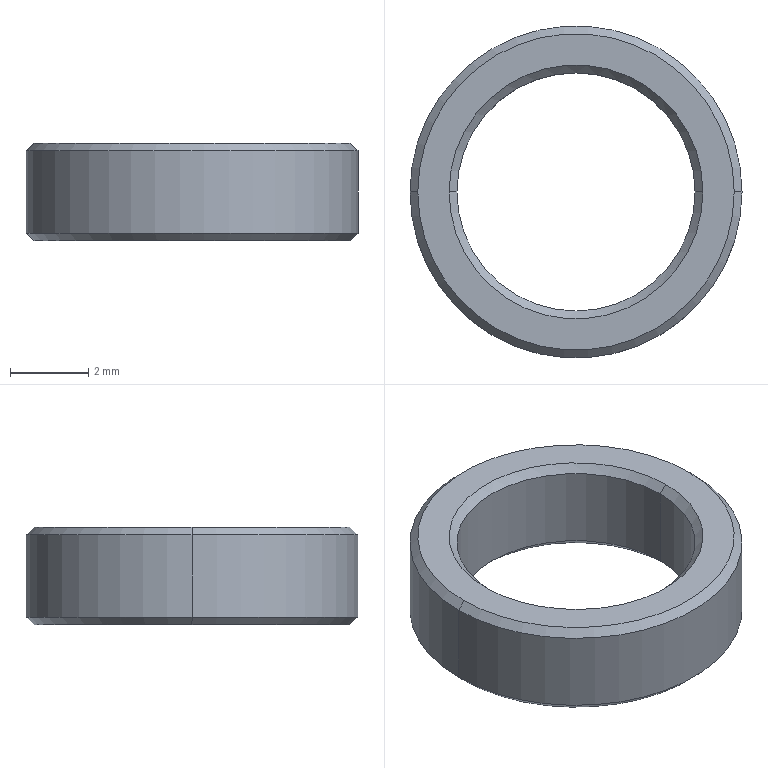Part | NX | features BREP 1 | 1 solid | 14 faces | box 8.5 x 8.5 x 2.5 mm | volume 66.966 mm3 | cone 8 | cylinder 4 | plane 2 | commonest cylinder face diameters 6.1 x2 8.5 x2
STEP:
#1=CARTESIAN_POINT('',(-3.25,0.,2.5));
#2=VERTEX_POINT('',#1);
#3=CARTESIAN_POINT('',(-3.05,0.,2.3));
#4=VERTEX_POINT('',#3);
#5=CARTESIAN_POINT('',(-3.05,0.,2.3));
#6=DIRECTION('',(-0.7071,0.,0.7071));
#7=VECTOR('',#6,1000.);
#8=LINE('',#5,#7);
#9=EDGE_CURVE('',#2,#4,#8,.F.);
#10=ORIENTED_EDGE('',*,*,#9,.T.);
#11=CARTESIAN_POINT('',(3.05,0.,2.3));
#12=VERTEX_POINT('',#11);
#13=CARTESIAN_POINT('',(0.,0.,2.3));
#14=DIRECTION('',(0.,0.,1.));
#15=DIRECTION('',(1.,0.,0.));
#16=AXIS2_PLACEMENT_3D('',#13,#14,#15);
#17=CIRCLE('',#16,3.05);
#18=EDGE_CURVE('',#12,#4,#17,.T.);
#19=ORIENTED_EDGE('',*,*,#18,.F.);
#20=CARTESIAN_POINT('',(3.25,0.,2.5));
#21=VERTEX_POINT('',#20);
#22=CARTESIAN_POINT('',(3.05,0.,2.3));
#23=DIRECTION('',(0.7071,0.,0.7071));
#24=VECTOR('',#23,1000.);
#25=LINE('',#22,#24);
#26=EDGE_CURVE('',#21,#12,#25,.F.);
#27=ORIENTED_EDGE('',*,*,#26,.F.);
#28=CARTESIAN_POINT('',(0.,0.,2.5));
#29=DIRECTION('',(0.,0.,-1.));
#30=DIRECTION('',(1.,0.,0.));
#31=AXIS2_PLACEMENT_3D('',#28,#29,#30);
#32=CIRCLE('',#31,3.25);
#33=EDGE_CURVE('',#2,#21,#32,.T.);
#34=ORIENTED_EDGE('',*,*,#33,.F.);
#35=EDGE_LOOP('',(#10,#19,#27,#34));
#36=FACE_BOUND('',#35,.T.);
#37=CARTESIAN_POINT('',(0.,0.,2.3));
#38=DIRECTION('',(0.,0.,1.));
#39=DIRECTION('',(1.,0.,0.));
#40=AXIS2_PLACEMENT_3D('',#37,#38,#39);
#41=CONICAL_SURFACE('',#40,3.05,0.7854);
#42=ADVANCED_FACE('',(#36),#41,.F.);
#43=CARTESIAN_POINT('',(3.05,0.,0.2));
#44=VERTEX_POINT('',#43);
#45=CARTESIAN_POINT('',(3.25,0.,0.));
#46=VERTEX_POINT('',#45);
#47=CARTESIAN_POINT('',(3.25,0.,0.));
#48=DIRECTION('',(0.7071,0.,-0.7071));
#49=VECTOR('',#48,1000.);
#50=LINE('',#47,#49);
#51=EDGE_CURVE('',#44,#46,#50,.T.);
#52=ORIENTED_EDGE('',*,*,#51,.F.);
#53=CARTESIAN_POINT('',(-3.05,0.,0.2));
#54=VERTEX_POINT('',#53);
#55=CARTESIAN_POINT('',(0.,0.,0.2));
#56=DIRECTION('',(0.,0.,-1.));
#57=DIRECTION('',(1.,0.,0.));
#58=AXIS2_PLACEMENT_3D('',#55,#56,#57);
#59=CIRCLE('',#58,3.05);
#60=EDGE_CURVE('',#54,#44,#59,.T.);
#61=ORIENTED_EDGE('',*,*,#60,.F.);
#62=CARTESIAN_POINT('',(-3.25,0.,0.));
#63=VERTEX_POINT('',#62);
#64=CARTESIAN_POINT('',(-3.25,0.,0.));
#65=DIRECTION('',(-0.7071,0.,-0.7071));
#66=VECTOR('',#65,1000.);
#67=LINE('',#64,#66);
#68=EDGE_CURVE('',#54,#63,#67,.T.);
#69=ORIENTED_EDGE('',*,*,#68,.T.);
#70=CARTESIAN_POINT('',(0.,0.,0.));
#71=DIRECTION('',(0.,0.,1.));
#72=DIRECTION('',(1.,0.,0.));
#73=AXIS2_PLACEMENT_3D('',#70,#71,#72);
#74=CIRCLE('',#73,3.25);
#75=EDGE_CURVE('',#46,#63,#74,.T.);
#76=ORIENTED_EDGE('',*,*,#75,.F.);
#77=EDGE_LOOP('',(#52,#61,#69,#76));
#78=FACE_BOUND('',#77,.T.);
#79=CARTESIAN_POINT('',(0.,0.,0.));
#80=DIRECTION('',(0.,0.,-1.));
#81=DIRECTION('',(-1.,0.,0.));
#82=AXIS2_PLACEMENT_3D('',#79,#80,#81);
#83=CONICAL_SURFACE('',#82,3.25,0.7854);
#84=ADVANCED_FACE('',(#78),#83,.F.);
#85=CARTESIAN_POINT('',(4.05,0.,2.5));
#86=VERTEX_POINT('',#85);
#87=CARTESIAN_POINT('',(4.25,0.,2.3));
#88=VERTEX_POINT('',#87);
#89=CARTESIAN_POINT('',(4.05,0.,2.5));
#90=DIRECTION('',(0.7071,0.,-0.7071));
#91=VECTOR('',#90,1000.);
#92=LINE('',#89,#91);
#93=EDGE_CURVE('',#86,#88,#92,.T.);
#94=ORIENTED_EDGE('',*,*,#93,.F.);
#95=CARTESIAN_POINT('',(-4.05,0.,2.5));
#96=VERTEX_POINT('',#95);
#97=CARTESIAN_POINT('',(0.,0.,2.5));
#98=DIRECTION('',(0.,0.,1.));
#99=DIRECTION('',(1.,0.,0.));
#100=AXIS2_PLACEMENT_3D('',#97,#98,#99);
#101=CIRCLE('',#100,4.05);
#102=EDGE_CURVE('',#96,#86,#101,.T.);
#103=ORIENTED_EDGE('',*,*,#102,.F.);
#104=CARTESIAN_POINT('',(-4.25,0.,2.3));
#105=VERTEX_POINT('',#104);
#106=CARTESIAN_POINT('',(-4.05,0.,2.5));
#107=DIRECTION('',(-0.7071,0.,-0.7071));
#108=VECTOR('',#107,1000.);
#109=LINE('',#106,#108);
#110=EDGE_CURVE('',#96,#105,#109,.T.);
#111=ORIENTED_EDGE('',*,*,#110,.T.);
#112=CARTESIAN_POINT('',(0.,0.,2.3));
#113=DIRECTION('',(0.,0.,-1.));
#114=DIRECTION('',(1.,0.,0.));
#115=AXIS2_PLACEMENT_3D('',#112,#113,#114);
#116=CIRCLE('',#115,4.25);
#117=EDGE_CURVE('',#88,#105,#116,.T.);
#118=ORIENTED_EDGE('',*,*,#117,.F.);
#119=EDGE_LOOP('',(#94,#103,#111,#118));
#120=FACE_BOUND('',#119,.T.);
#121=CARTESIAN_POINT('',(0.,0.,2.5));
#122=DIRECTION('',(0.,0.,-1.));
#123=DIRECTION('',(-1.,0.,0.));
#124=AXIS2_PLACEMENT_3D('',#121,#122,#123);
#125=CONICAL_SURFACE('',#124,4.05,0.7854);
#126=ADVANCED_FACE('',(#120),#125,.T.);
#127=CARTESIAN_POINT('',(-4.25,0.,0.2));
#128=VERTEX_POINT('',#127);
#129=CARTESIAN_POINT('',(-4.05,0.,0.));
#130=VERTEX_POINT('',#129);
#131=CARTESIAN_POINT('',(-4.25,0.,0.2));
#132=DIRECTION('',(-0.7071,0.,0.7071));
#133=VECTOR('',#132,1000.);
#134=LINE('',#131,#133);
#135=EDGE_CURVE('',#128,#130,#134,.F.);
#136=ORIENTED_EDGE('',*,*,#135,.T.);
#137=CARTESIAN_POINT('',(4.05,0.,0.));
#138=VERTEX_POINT('',#137);
#139=CARTESIAN_POINT('',(0.,0.,0.));
#140=DIRECTION('',(0.,0.,-1.));
#141=DIRECTION('',(1.,0.,0.));
#142=AXIS2_PLACEMENT_3D('',#139,#140,#141);
#143=CIRCLE('',#142,4.05);
#144=EDGE_CURVE('',#138,#130,#143,.T.);
#145=ORIENTED_EDGE('',*,*,#144,.F.);
#146=CARTESIAN_POINT('',(4.25,0.,0.2));
#147=VERTEX_POINT('',#146);
#148=CARTESIAN_POINT('',(4.25,0.,0.2));
#149=DIRECTION('',(0.7071,0.,0.7071));
#150=VECTOR('',#149,1000.);
#151=LINE('',#148,#150);
#152=EDGE_CURVE('',#147,#138,#151,.F.);
#153=ORIENTED_EDGE('',*,*,#152,.F.);
#154=CARTESIAN_POINT('',(0.,0.,0.2));
#155=DIRECTION('',(0.,0.,1.));
#156=DIRECTION('',(1.,0.,0.));
#157=AXIS2_PLACEMENT_3D('',#154,#155,#156);
#158=CIRCLE('',#157,4.25);
#159=EDGE_CURVE('',#128,#147,#158,.T.);
#160=ORIENTED_EDGE('',*,*,#159,.F.);
#161=EDGE_LOOP('',(#136,#145,#153,#160));
#162=FACE_BOUND('',#161,.T.);
#163=CARTESIAN_POINT('',(0.,0.,0.2));
#164=DIRECTION('',(0.,0.,1.));
#165=DIRECTION('',(1.,0.,0.));
#166=AXIS2_PLACEMENT_3D('',#163,#164,#165);
#167=CONICAL_SURFACE('',#166,4.25,0.7854);
#168=ADVANCED_FACE('',(#162),#167,.T.);
#169=CARTESIAN_POINT('',(3.05,0.,2.5));
#170=DIRECTION('',(0.,0.,-1.));
#171=VECTOR('',#170,1000.);
#172=LINE('',#169,#171);
#173=EDGE_CURVE('',#12,#44,#172,.T.);
#174=ORIENTED_EDGE('',*,*,#173,.F.);
#175=ORIENTED_EDGE('',*,*,#18,.T.);
#176=CARTESIAN_POINT('',(-3.05,0.,2.5));
#177=DIRECTION('',(0.,0.,-1.));
#178=VECTOR('',#177,1000.);
#179=LINE('',#176,#178);
#180=EDGE_CURVE('',#4,#54,#179,.T.);
#181=ORIENTED_EDGE('',*,*,#180,.T.);
#182=ORIENTED_EDGE('',*,*,#60,.T.);
#183=EDGE_LOOP('',(#174,#175,#181,#182));
#184=FACE_BOUND('',#183,.T.);
#185=CARTESIAN_POINT('',(0.,0.,2.5));
#186=DIRECTION('',(0.,0.,-1.));
#187=DIRECTION('',(-1.,0.,0.));
#188=AXIS2_PLACEMENT_3D('',#185,#186,#187);
#189=CYLINDRICAL_SURFACE('',#188,3.05);
#190=ADVANCED_FACE('',(#184),#189,.F.);
#191=CARTESIAN_POINT('',(4.25,0.,2.5));
#192=DIRECTION('',(0.,0.,-1.));
#193=VECTOR('',#192,1000.);
#194=LINE('',#191,#193);
#195=EDGE_CURVE('',#88,#147,#194,.T.);
#196=ORIENTED_EDGE('',*,*,#195,.F.);
#197=ORIENTED_EDGE('',*,*,#117,.T.);
#198=CARTESIAN_POINT('',(-4.25,0.,2.5));
#199=DIRECTION('',(0.,0.,-1.));
#200=VECTOR('',#199,1000.);
#201=LINE('',#198,#200);
#202=EDGE_CURVE('',#105,#128,#201,.T.);
#203=ORIENTED_EDGE('',*,*,#202,.T.);
#204=ORIENTED_EDGE('',*,*,#159,.T.);
#205=EDGE_LOOP('',(#196,#197,#203,#204));
#206=FACE_BOUND('',#205,.T.);
#207=CARTESIAN_POINT('',(0.,0.,2.5));
#208=DIRECTION('',(0.,0.,-1.));
#209=DIRECTION('',(-1.,0.,0.));
#210=AXIS2_PLACEMENT_3D('',#207,#208,#209);
#211=CYLINDRICAL_SURFACE('',#210,4.25);
#212=ADVANCED_FACE('',(#206),#211,.T.);
#213=CARTESIAN_POINT('',(0.,0.,0.));
#214=DIRECTION('',(0.,0.,1.));
#215=DIRECTION('',(1.,0.,0.));
#216=AXIS2_PLACEMENT_3D('',#213,#214,#215);
#217=CIRCLE('',#216,3.25);
#218=EDGE_CURVE('',#63,#46,#217,.T.);
#219=ORIENTED_EDGE('',*,*,#218,.T.);
#220=ORIENTED_EDGE('',*,*,#75,.T.);
#221=EDGE_LOOP('',(#219,#220));
#222=FACE_BOUND('',#221,.T.);
#223=ORIENTED_EDGE('',*,*,#144,.T.);
#224=CARTESIAN_POINT('',(0.,0.,0.));
#225=DIRECTION('',(0.,0.,-1.));
#226=DIRECTION('',(1.,0.,0.));
#227=AXIS2_PLACEMENT_3D('',#224,#225,#226);
#228=CIRCLE('',#227,4.05);
#229=EDGE_CURVE('',#130,#138,#228,.T.);
#230=ORIENTED_EDGE('',*,*,#229,.T.);
#231=EDGE_LOOP('',(#223,#230));
#232=FACE_BOUND('',#231,.T.);
#233=CARTESIAN_POINT('',(0.,0.,0.));
#234=DIRECTION('',(0.,0.,1.));
#235=DIRECTION('',(1.,0.,0.));
#236=AXIS2_PLACEMENT_3D('',#233,#234,#235);
#237=PLANE('',#236);
#238=ADVANCED_FACE('',(#222,#232),#237,.F.);
#239=CARTESIAN_POINT('',(0.,0.,2.5));
#240=DIRECTION('',(0.,0.,-1.));
#241=DIRECTION('',(1.,0.,0.));
#242=AXIS2_PLACEMENT_3D('',#239,#240,#241);
#243=CIRCLE('',#242,3.25);
#244=EDGE_CURVE('',#21,#2,#243,.T.);
#245=ORIENTED_EDGE('',*,*,#244,.T.);
#246=ORIENTED_EDGE('',*,*,#33,.T.);
#247=EDGE_LOOP('',(#245,#246));
#248=FACE_BOUND('',#247,.T.);
#249=ORIENTED_EDGE('',*,*,#102,.T.);
#250=CARTESIAN_POINT('',(0.,0.,2.5));
#251=DIRECTION('',(0.,0.,1.));
#252=DIRECTION('',(1.,0.,0.));
#253=AXIS2_PLACEMENT_3D('',#250,#251,#252);
#254=CIRCLE('',#253,4.05);
#255=EDGE_CURVE('',#86,#96,#254,.T.);
#256=ORIENTED_EDGE('',*,*,#255,.T.);
#257=EDGE_LOOP('',(#249,#256));
#258=FACE_BOUND('',#257,.T.);
#259=CARTESIAN_POINT('',(0.,0.,2.5));
#260=DIRECTION('',(0.,0.,1.));
#261=DIRECTION('',(1.,0.,0.));
#262=AXIS2_PLACEMENT_3D('',#259,#260,#261);
#263=PLANE('',#262);
#264=ADVANCED_FACE('',(#248,#258),#263,.T.);
#265=CARTESIAN_POINT('',(0.,0.,2.3));
#266=DIRECTION('',(0.,0.,-1.));
#267=DIRECTION('',(1.,0.,0.));
#268=AXIS2_PLACEMENT_3D('',#265,#266,#267);
#269=CIRCLE('',#268,4.25);
#270=EDGE_CURVE('',#105,#88,#269,.T.);
#271=ORIENTED_EDGE('',*,*,#270,.T.);
#272=ORIENTED_EDGE('',*,*,#195,.T.);
#273=CARTESIAN_POINT('',(0.,0.,0.2));
#274=DIRECTION('',(0.,0.,1.));
#275=DIRECTION('',(1.,0.,0.));
#276=AXIS2_PLACEMENT_3D('',#273,#274,#275);
#277=CIRCLE('',#276,4.25);
#278=EDGE_CURVE('',#147,#128,#277,.T.);
#279=ORIENTED_EDGE('',*,*,#278,.T.);
#280=ORIENTED_EDGE('',*,*,#202,.F.);
#281=EDGE_LOOP('',(#271,#272,#279,#280));
#282=FACE_BOUND('',#281,.T.);
#283=CARTESIAN_POINT('',(0.,0.,2.5));
#284=DIRECTION('',(0.,0.,-1.));
#285=DIRECTION('',(-1.,0.,0.));
#286=AXIS2_PLACEMENT_3D('',#283,#284,#285);
#287=CYLINDRICAL_SURFACE('',#286,4.25);
#288=ADVANCED_FACE('',(#282),#287,.T.);
#289=CARTESIAN_POINT('',(0.,0.,2.3));
#290=DIRECTION('',(0.,0.,1.));
#291=DIRECTION('',(1.,0.,0.));
#292=AXIS2_PLACEMENT_3D('',#289,#290,#291);
#293=CIRCLE('',#292,3.05);
#294=EDGE_CURVE('',#4,#12,#293,.T.);
#295=ORIENTED_EDGE('',*,*,#294,.T.);
#296=ORIENTED_EDGE('',*,*,#173,.T.);
#297=CARTESIAN_POINT('',(0.,0.,0.2));
#298=DIRECTION('',(0.,0.,-1.));
#299=DIRECTION('',(1.,0.,0.));
#300=AXIS2_PLACEMENT_3D('',#297,#298,#299);
#301=CIRCLE('',#300,3.05);
#302=EDGE_CURVE('',#44,#54,#301,.T.);
#303=ORIENTED_EDGE('',*,*,#302,.T.);
#304=ORIENTED_EDGE('',*,*,#180,.F.);
#305=EDGE_LOOP('',(#295,#296,#303,#304));
#306=FACE_BOUND('',#305,.T.);
#307=CARTESIAN_POINT('',(0.,0.,2.5));
#308=DIRECTION('',(0.,0.,-1.));
#309=DIRECTION('',(-1.,0.,0.));
#310=AXIS2_PLACEMENT_3D('',#307,#308,#309);
#311=CYLINDRICAL_SURFACE('',#310,3.05);
#312=ADVANCED_FACE('',(#306),#311,.F.);
#313=ORIENTED_EDGE('',*,*,#229,.F.);
#314=ORIENTED_EDGE('',*,*,#135,.F.);
#315=ORIENTED_EDGE('',*,*,#278,.F.);
#316=ORIENTED_EDGE('',*,*,#152,.T.);
#317=EDGE_LOOP('',(#313,#314,#315,#316));
#318=FACE_BOUND('',#317,.T.);
#319=CARTESIAN_POINT('',(0.,0.,0.2));
#320=DIRECTION('',(0.,0.,1.));
#321=DIRECTION('',(1.,0.,0.));
#322=AXIS2_PLACEMENT_3D('',#319,#320,#321);
#323=CONICAL_SURFACE('',#322,4.25,0.7854);
#324=ADVANCED_FACE('',(#318),#323,.T.);
#325=ORIENTED_EDGE('',*,*,#255,.F.);
#326=ORIENTED_EDGE('',*,*,#93,.T.);
#327=ORIENTED_EDGE('',*,*,#270,.F.);
#328=ORIENTED_EDGE('',*,*,#110,.F.);
#329=EDGE_LOOP('',(#325,#326,#327,#328));
#330=FACE_BOUND('',#329,.T.);
#331=CARTESIAN_POINT('',(0.,0.,2.5));
#332=DIRECTION('',(0.,0.,-1.));
#333=DIRECTION('',(-1.,0.,0.));
#334=AXIS2_PLACEMENT_3D('',#331,#332,#333);
#335=CONICAL_SURFACE('',#334,4.05,0.7854);
#336=ADVANCED_FACE('',(#330),#335,.T.);
#337=ORIENTED_EDGE('',*,*,#302,.F.);
#338=ORIENTED_EDGE('',*,*,#51,.T.);
#339=ORIENTED_EDGE('',*,*,#218,.F.);
#340=ORIENTED_EDGE('',*,*,#68,.F.);
#341=EDGE_LOOP('',(#337,#338,#339,#340));
#342=FACE_BOUND('',#341,.T.);
#343=CARTESIAN_POINT('',(0.,0.,0.));
#344=DIRECTION('',(0.,0.,-1.));
#345=DIRECTION('',(-1.,0.,0.));
#346=AXIS2_PLACEMENT_3D('',#343,#344,#345);
#347=CONICAL_SURFACE('',#346,3.25,0.7854);
#348=ADVANCED_FACE('',(#342),#347,.F.);
#349=ORIENTED_EDGE('',*,*,#294,.F.);
#350=ORIENTED_EDGE('',*,*,#9,.F.);
#351=ORIENTED_EDGE('',*,*,#244,.F.);
#352=ORIENTED_EDGE('',*,*,#26,.T.);
#353=EDGE_LOOP('',(#349,#350,#351,#352));
#354=FACE_BOUND('',#353,.T.);
#355=CARTESIAN_POINT('',(0.,0.,2.3));
#356=DIRECTION('',(0.,0.,1.));
#357=DIRECTION('',(1.,0.,0.));
#358=AXIS2_PLACEMENT_3D('',#355,#356,#357);
#359=CONICAL_SURFACE('',#358,3.05,0.7854);
#360=ADVANCED_FACE('',(#354),#359,.F.);
#361=CLOSED_SHELL('',(#42,#84,#126,#168,#190,#212,#238,#264,#288,#312,#324,#336,#348,#360));
#362=MANIFOLD_SOLID_BREP('',#361);
#363=(LENGTH_UNIT()NAMED_UNIT(*)SI_UNIT(.MILLI.,.METRE.));
#364=UNCERTAINTY_MEASURE_WITH_UNIT(LENGTH_MEASURE(0.00001),#363,'','');
#365=(NAMED_UNIT(*)PLANE_ANGLE_UNIT()SI_UNIT($,.RADIAN.));
#366=(NAMED_UNIT(*)SI_UNIT($,.STERADIAN.)SOLID_ANGLE_UNIT());
#367=(GEOMETRIC_REPRESENTATION_CONTEXT(3)GLOBAL_UNCERTAINTY_ASSIGNED_CONTEXT((#364))GLOBAL_UNIT_ASSIGNED_CONTEXT((#363,#365,#366))REPRESENTATION_CONTEXT('',''));
#368=ADVANCED_BREP_SHAPE_REPRESENTATION('',(#362),#367);